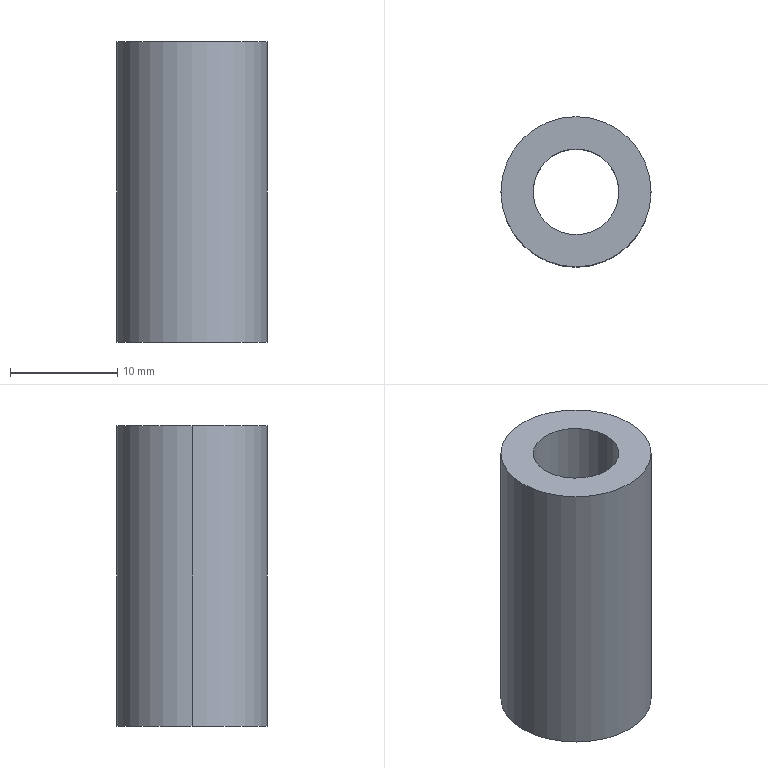Part | SolidWorks | features Extrusion 1 | 1 solid | 6 faces | box 14 x 14 x 28 mm | volume 2903 mm3 | cylinder 4 | plane 2 | commonest cylinder face diameters 8 x2 14 x2
STEP:
#1=CARTESIAN_POINT('',(-4.,0.,-28.));
#2=VERTEX_POINT('',#1);
#3=CARTESIAN_POINT('',(4.,0.,-28.));
#4=VERTEX_POINT('',#3);
#5=CARTESIAN_POINT('',(0.,0.,-28.));
#6=DIRECTION('',(0.,0.,1.));
#7=DIRECTION('',(1.,0.,0.));
#8=AXIS2_PLACEMENT_3D('',#5,#6,#7);
#9=CIRCLE('',#8,4.);
#10=EDGE_CURVE('',#2,#4,#9,.T.);
#11=ORIENTED_EDGE('',*,*,#10,.F.);
#12=CARTESIAN_POINT('',(-4.,0.,0.));
#13=VERTEX_POINT('',#12);
#14=CARTESIAN_POINT('',(-4.,0.,-28.));
#15=DIRECTION('',(0.,0.,1.));
#16=VECTOR('',#15,1000.);
#17=LINE('',#14,#16);
#18=EDGE_CURVE('',#2,#13,#17,.T.);
#19=ORIENTED_EDGE('',*,*,#18,.T.);
#20=CARTESIAN_POINT('',(4.,0.,0.));
#21=VERTEX_POINT('',#20);
#22=CARTESIAN_POINT('',(0.,0.,0.));
#23=DIRECTION('',(0.,0.,1.));
#24=DIRECTION('',(1.,0.,0.));
#25=AXIS2_PLACEMENT_3D('',#22,#23,#24);
#26=CIRCLE('',#25,4.);
#27=EDGE_CURVE('',#13,#21,#26,.T.);
#28=ORIENTED_EDGE('',*,*,#27,.T.);
#29=CARTESIAN_POINT('',(4.,0.,-28.));
#30=DIRECTION('',(0.,0.,1.));
#31=VECTOR('',#30,1000.);
#32=LINE('',#29,#31);
#33=EDGE_CURVE('',#4,#21,#32,.T.);
#34=ORIENTED_EDGE('',*,*,#33,.F.);
#35=EDGE_LOOP('',(#11,#19,#28,#34));
#36=FACE_OUTER_BOUND('',#35,.T.);
#37=CARTESIAN_POINT('',(0.,0.,-28.));
#38=DIRECTION('',(0.,0.,1.));
#39=DIRECTION('',(1.,0.,0.));
#40=AXIS2_PLACEMENT_3D('',#37,#38,#39);
#41=CYLINDRICAL_SURFACE('',#40,4.);
#42=ADVANCED_FACE('',(#36),#41,.F.);
#43=CARTESIAN_POINT('',(7.,0.,-28.));
#44=VERTEX_POINT('',#43);
#45=CARTESIAN_POINT('',(-7.,0.,-28.));
#46=VERTEX_POINT('',#45);
#47=CARTESIAN_POINT('',(0.,0.,-28.));
#48=DIRECTION('',(0.,0.,1.));
#49=DIRECTION('',(1.,0.,0.));
#50=AXIS2_PLACEMENT_3D('',#47,#48,#49);
#51=CIRCLE('',#50,7.);
#52=EDGE_CURVE('',#44,#46,#51,.T.);
#53=ORIENTED_EDGE('',*,*,#52,.T.);
#54=CARTESIAN_POINT('',(-7.,0.,0.));
#55=VERTEX_POINT('',#54);
#56=CARTESIAN_POINT('',(-7.,0.,-28.));
#57=DIRECTION('',(0.,0.,1.));
#58=VECTOR('',#57,1000.);
#59=LINE('',#56,#58);
#60=EDGE_CURVE('',#46,#55,#59,.T.);
#61=ORIENTED_EDGE('',*,*,#60,.T.);
#62=CARTESIAN_POINT('',(7.,0.,0.));
#63=VERTEX_POINT('',#62);
#64=CARTESIAN_POINT('',(0.,0.,0.));
#65=DIRECTION('',(0.,0.,1.));
#66=DIRECTION('',(1.,0.,0.));
#67=AXIS2_PLACEMENT_3D('',#64,#65,#66);
#68=CIRCLE('',#67,7.);
#69=EDGE_CURVE('',#63,#55,#68,.T.);
#70=ORIENTED_EDGE('',*,*,#69,.F.);
#71=CARTESIAN_POINT('',(7.,0.,-28.));
#72=DIRECTION('',(0.,0.,1.));
#73=VECTOR('',#72,1000.);
#74=LINE('',#71,#73);
#75=EDGE_CURVE('',#44,#63,#74,.T.);
#76=ORIENTED_EDGE('',*,*,#75,.F.);
#77=EDGE_LOOP('',(#53,#61,#70,#76));
#78=FACE_OUTER_BOUND('',#77,.T.);
#79=CARTESIAN_POINT('',(0.,0.,-28.));
#80=DIRECTION('',(0.,0.,1.));
#81=DIRECTION('',(1.,0.,0.));
#82=AXIS2_PLACEMENT_3D('',#79,#80,#81);
#83=CYLINDRICAL_SURFACE('',#82,7.);
#84=ADVANCED_FACE('',(#78),#83,.T.);
#85=ORIENTED_EDGE('',*,*,#60,.F.);
#86=CARTESIAN_POINT('',(0.,0.,-28.));
#87=DIRECTION('',(0.,0.,1.));
#88=DIRECTION('',(1.,0.,0.));
#89=AXIS2_PLACEMENT_3D('',#86,#87,#88);
#90=CIRCLE('',#89,7.);
#91=EDGE_CURVE('',#46,#44,#90,.T.);
#92=ORIENTED_EDGE('',*,*,#91,.T.);
#93=ORIENTED_EDGE('',*,*,#75,.T.);
#94=CARTESIAN_POINT('',(0.,0.,0.));
#95=DIRECTION('',(0.,0.,1.));
#96=DIRECTION('',(1.,0.,0.));
#97=AXIS2_PLACEMENT_3D('',#94,#95,#96);
#98=CIRCLE('',#97,7.);
#99=EDGE_CURVE('',#55,#63,#98,.T.);
#100=ORIENTED_EDGE('',*,*,#99,.F.);
#101=EDGE_LOOP('',(#85,#92,#93,#100));
#102=FACE_OUTER_BOUND('',#101,.T.);
#103=CARTESIAN_POINT('',(0.,0.,-28.));
#104=DIRECTION('',(0.,0.,1.));
#105=DIRECTION('',(1.,0.,0.));
#106=AXIS2_PLACEMENT_3D('',#103,#104,#105);
#107=CYLINDRICAL_SURFACE('',#106,7.);
#108=ADVANCED_FACE('',(#102),#107,.T.);
#109=CARTESIAN_POINT('',(0.,0.,-28.));
#110=DIRECTION('',(0.,0.,1.));
#111=DIRECTION('',(1.,0.,0.));
#112=AXIS2_PLACEMENT_3D('',#109,#110,#111);
#113=CIRCLE('',#112,4.);
#114=EDGE_CURVE('',#4,#2,#113,.T.);
#115=ORIENTED_EDGE('',*,*,#114,.T.);
#116=ORIENTED_EDGE('',*,*,#10,.T.);
#117=EDGE_LOOP('',(#115,#116));
#118=FACE_BOUND('',#117,.T.);
#119=ORIENTED_EDGE('',*,*,#52,.F.);
#120=ORIENTED_EDGE('',*,*,#91,.F.);
#121=EDGE_LOOP('',(#119,#120));
#122=FACE_OUTER_BOUND('',#121,.T.);
#123=CARTESIAN_POINT('',(0.,0.,-28.));
#124=DIRECTION('',(0.,0.,1.));
#125=DIRECTION('',(1.,0.,0.));
#126=AXIS2_PLACEMENT_3D('',#123,#124,#125);
#127=PLANE('',#126);
#128=ADVANCED_FACE('',(#118,#122),#127,.F.);
#129=CARTESIAN_POINT('',(0.,0.,0.));
#130=DIRECTION('',(0.,0.,1.));
#131=DIRECTION('',(1.,0.,0.));
#132=AXIS2_PLACEMENT_3D('',#129,#130,#131);
#133=CIRCLE('',#132,4.);
#134=EDGE_CURVE('',#21,#13,#133,.T.);
#135=ORIENTED_EDGE('',*,*,#134,.F.);
#136=ORIENTED_EDGE('',*,*,#27,.F.);
#137=EDGE_LOOP('',(#135,#136));
#138=FACE_BOUND('',#137,.T.);
#139=ORIENTED_EDGE('',*,*,#69,.T.);
#140=ORIENTED_EDGE('',*,*,#99,.T.);
#141=EDGE_LOOP('',(#139,#140));
#142=FACE_OUTER_BOUND('',#141,.T.);
#143=CARTESIAN_POINT('',(0.,0.,0.));
#144=DIRECTION('',(0.,0.,1.));
#145=DIRECTION('',(1.,0.,0.));
#146=AXIS2_PLACEMENT_3D('',#143,#144,#145);
#147=PLANE('',#146);
#148=ADVANCED_FACE('',(#138,#142),#147,.T.);
#149=ORIENTED_EDGE('',*,*,#18,.F.);
#150=ORIENTED_EDGE('',*,*,#114,.F.);
#151=ORIENTED_EDGE('',*,*,#33,.T.);
#152=ORIENTED_EDGE('',*,*,#134,.T.);
#153=EDGE_LOOP('',(#149,#150,#151,#152));
#154=FACE_OUTER_BOUND('',#153,.T.);
#155=CARTESIAN_POINT('',(0.,0.,-28.));
#156=DIRECTION('',(0.,0.,1.));
#157=DIRECTION('',(1.,0.,0.));
#158=AXIS2_PLACEMENT_3D('',#155,#156,#157);
#159=CYLINDRICAL_SURFACE('',#158,4.);
#160=ADVANCED_FACE('',(#154),#159,.F.);
#161=CLOSED_SHELL('',(#42,#84,#108,#128,#148,#160));
#162=MANIFOLD_SOLID_BREP('',#161);
#163=CARTESIAN_POINT('',(0.,0.,0.));
#164=DIRECTION('',(0.,0.,1.));
#165=DIRECTION('',(1.,0.,0.));
#166=AXIS2_PLACEMENT_3D('',#163,#164,#165);
#167=(LENGTH_UNIT()NAMED_UNIT(*)SI_UNIT(.MILLI.,.METRE.));
#168=UNCERTAINTY_MEASURE_WITH_UNIT(LENGTH_MEASURE(0.00001),#167,'','');
#169=(NAMED_UNIT(*)PLANE_ANGLE_UNIT()SI_UNIT($,.RADIAN.));
#170=(NAMED_UNIT(*)SI_UNIT($,.STERADIAN.)SOLID_ANGLE_UNIT());
#171=(GEOMETRIC_REPRESENTATION_CONTEXT(3)GLOBAL_UNCERTAINTY_ASSIGNED_CONTEXT((#168))GLOBAL_UNIT_ASSIGNED_CONTEXT((#167,#169,#170))REPRESENTATION_CONTEXT('',''));
#172=ADVANCED_BREP_SHAPE_REPRESENTATION('',(#162,#166),#171);